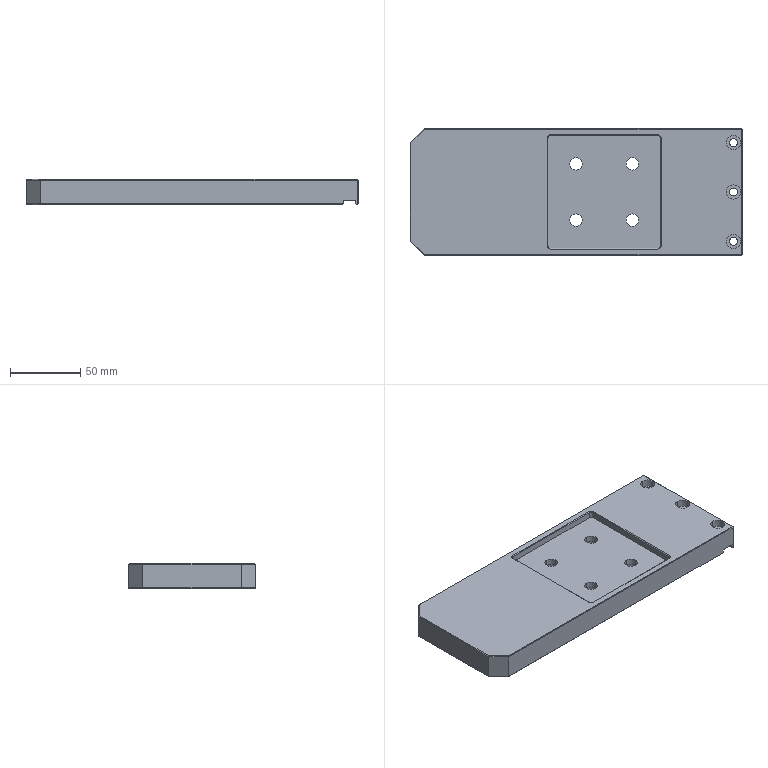NC program | NX | posted with a generic post | part box 235.5 x 90 x 18 mm
Lines 1609 to 2446 of 2446:
(ZLEVEL_PROFILE_COPY_1 , TOOL : D4)
N3186 T11 M6
N3188 G54
N3190 G17 G0 G90 X54.41 Y-37.2 S9500 M3
N3192 G43 Z30. H11
N3194 Z-0.769
N3196 G94 G1 X54.757 Y-37.8 F1000.
N3198 G3 X55.103 Y-38. R0.4
N3200 G1 X58. F2000.
N3202 Y-35.103
N3204 G3 X57.8 Y-34.757 R0.4
N3206 G1 X57.2 Y-34.41
N3208 G0 X54.41 Y-37.2 Z-1.154
N3210 G1 X54.757 Y-37.8 F1000.
N3212 G3 X55.103 Y-38. R0.4
N3214 G1 X58. F2000.
N3216 Y-35.103
N3218 G3 X57.8 Y-34.757 R0.4
N3220 G1 X57.2 Y-34.41
N3222 G0 X54.41 Y-37.2 Z-1.538
N3224 G1 X54.757 Y-37.8 F1000.
N3226 G3 X55.103 Y-38. R0.4
N3228 G1 X58. F2000.
N3230 Y-35.103
N3232 G3 X57.8 Y-34.757 R0.4
N3234 G1 X57.2 Y-34.41
N3236 G0 X54.41 Y-37.2 Z-1.923
N3238 G1 X54.757 Y-37.8 F1000.
N3240 G3 X55.103 Y-38. R0.4
N3242 G1 X58. F2000.
N3244 Y-35.103
N3246 G3 X57.8 Y-34.757 R0.4
N3248 G1 X57.2 Y-34.41
N3250 G0 X54.41 Y-37.2 Z-2.308
N3252 G1 X54.757 Y-37.8 F1000.
N3254 G3 X55.103 Y-38. R0.4
N3256 G1 X58. F2000.
N3258 Y-35.103
N3260 G3 X57.8 Y-34.757 R0.4
N3262 G1 X57.2 Y-34.41
N3264 G0 X54.41 Y-37.2 Z-2.692
N3266 G1 X54.757 Y-37.8 F1000.
N3268 G3 X55.103 Y-38. R0.4
N3270 G1 X58. F2000.
N3272 Y-35.103
N3274 G3 X57.8 Y-34.757 R0.4
N3276 G1 X57.2 Y-34.41
N3278 G0 X54.41 Y-37.2 Z-3.077
N3280 G1 X54.757 Y-37.8 F1000.
N3282 G3 X55.103 Y-38. R0.4
N3284 G1 X58. F2000.
N3286 Y-35.103
N3288 G3 X57.8 Y-34.757 R0.4
N3290 G1 X57.2 Y-34.41
N3292 G0 X54.41 Y-37.2 Z-3.462
N3294 G1 X54.757 Y-37.8 F1000.
N3296 G3 X55.103 Y-38. R0.4
N3298 G1 X58. F2000.
N3300 Y-35.103
N3302 G3 X57.8 Y-34.757 R0.4
N3304 G1 X57.2 Y-34.41
N3306 G0 X54.41 Y-37.2 Z-3.846
N3308 G1 X54.757 Y-37.8 F1000.
N3310 G3 X55.103 Y-38. R0.4
N3312 G1 X58. F2000.
N3314 Y-35.103
N3316 G3 X57.8 Y-34.757 R0.4
N3318 G1 X57.2 Y-34.41
N3320 G0 X54.41 Y-37.2 Z-4.231
N3322 G1 X54.757 Y-37.8 F1000.
N3324 G3 X55.103 Y-38. R0.4
N3326 G1 X58. F2000.
N3328 Y-35.103
N3330 G3 X57.8 Y-34.757 R0.4
N3332 G1 X57.2 Y-34.41
N3334 G0 X54.41 Y-37.2 Z-4.615
N3336 G1 X54.757 Y-37.8 F1000.
N3338 G3 X55.103 Y-38. R0.4
N3340 G1 X58. F2000.
N3342 Y-35.103
N3344 G3 X57.8 Y-34.757 R0.4
N3346 G1 X57.2 Y-34.41
N3348 G0 X54.41 Y-37.2 Z-5.
N3350 G1 X54.757 Y-37.8 F1000.
N3352 G3 X55.103 Y-38. R0.4
N3354 G1 X58. F2000.
N3356 Y-35.103
N3358 G3 X57.8 Y-34.757 R0.4
N3360 G1 X57.2 Y-34.41
N3362 G0 Z30.
N3364 Y34.41
N3366 Z-0.769
N3368 G1 X57.8 Y34.757 F1000.
N3370 G3 X58. Y35.103 R0.4
N3372 G1 Y38. F2000.
N3374 X55.103
N3376 G3 X54.757 Y37.8 R0.4
N3378 G1 X54.41 Y37.2
N3380 G0 X57.2 Y34.41 Z-1.154
N3382 G1 X57.8 Y34.757 F1000.
N3384 G3 X58. Y35.103 R0.4
N3386 G1 Y38. F2000.
N3388 X55.103
N3390 G3 X54.757 Y37.8 R0.4
N3392 G1 X54.41 Y37.2
N3394 G0 X57.2 Y34.41 Z-1.538
N3396 G1 X57.8 Y34.757 F1000.
N3398 G3 X58. Y35.103 R0.4
N3400 G1 Y38. F2000.
N3402 X55.103
N3404 G3 X54.757 Y37.8 R0.4
N3406 G1 X54.41 Y37.2
N3408 G0 X57.2 Y34.41 Z-1.923
N3410 G1 X57.8 Y34.757 F1000.
N3412 G3 X58. Y35.103 R0.4
N3414 G1 Y38. F2000.
N3416 X55.103
N3418 G3 X54.757 Y37.8 R0.4
N3420 G1 X54.41 Y37.2
N3422 G0 X57.2 Y34.41 Z-2.308
N3424 G1 X57.8 Y34.757 F1000.
N3426 G3 X58. Y35.103 R0.4
N3428 G1 Y38. F2000.
N3430 X55.103
N3432 G3 X54.757 Y37.8 R0.4
N3434 G1 X54.41 Y37.2
N3436 G0 X57.2 Y34.41 Z-2.692
N3438 G1 X57.8 Y34.757 F1000.
N3440 G3 X58. Y35.103 R0.4
N3442 G1 Y38. F2000.
N3444 X55.103
N3446 G3 X54.757 Y37.8 R0.4
N3448 G1 X54.41 Y37.2
N3450 G0 X57.2 Y34.41 Z-3.077
N3452 G1 X57.8 Y34.757 F1000.
N3454 G3 X58. Y35.103 R0.4
N3456 G1 Y38. F2000.
N3458 X55.103
N3460 G3 X54.757 Y37.8 R0.4
N3462 G1 X54.41 Y37.2
N3464 G0 X57.2 Y34.41 Z-3.462
N3466 G1 X57.8 Y34.757 F1000.
N3468 G3 X58. Y35.103 R0.4
N3470 G1 Y38. F2000.
N3472 X55.103
N3474 G3 X54.757 Y37.8 R0.4
N3476 G1 X54.41 Y37.2
N3478 G0 X57.2 Y34.41 Z-3.846
N3480 G1 X57.8 Y34.757 F1000.
N3482 G3 X58. Y35.103 R0.4
N3484 G1 Y38. F2000.
N3486 X55.103
N3488 G3 X54.757 Y37.8 R0.4
N3490 G1 X54.41 Y37.2
N3492 G0 X57.2 Y34.41 Z-4.231
N3494 G1 X57.8 Y34.757 F1000.
N3496 G3 X58. Y35.103 R0.4
N3498 G1 Y38. F2000.
N3500 X55.103
N3502 G3 X54.757 Y37.8 R0.4
N3504 G1 X54.41 Y37.2
N3506 G0 X57.2 Y34.41 Z-4.615
N3508 G1 X57.8 Y34.757 F1000.
N3510 G3 X58. Y35.103 R0.4
N3512 G1 Y38. F2000.
N3514 X55.103
N3516 G3 X54.757 Y37.8 R0.4
N3518 G1 X54.41 Y37.2
N3520 G0 X57.2 Y34.41 Z-5.
N3522 G1 X57.8 Y34.757 F1000.
N3524 G3 X58. Y35.103 R0.4
N3526 G1 Y38. F2000.
N3528 X55.103
N3530 G3 X54.757 Y37.8 R0.4
N3532 G1 X54.41 Y37.2
N3534 G0 Z30.
N3536 X-14.41
N3538 Z-0.769
N3540 G1 X-14.757 Y37.8 F1000.
N3542 G3 X-15.103 Y38. R0.4
N3544 G1 X-17.91 F2000.
N3546 X-18.
N3548 Y35.103
N3550 G3 X-17.8 Y34.757 R0.4
N3552 G1 X-17.2 Y34.41
N3554 G0 X-14.41 Y37.2 Z-1.154
N3556 G1 X-14.757 Y37.8 F1000.
N3558 G3 X-15.103 Y38. R0.4
N3560 G1 X-17.91 F2000.
N3562 X-18.
N3564 Y35.103
N3566 G3 X-17.8 Y34.757 R0.4
N3568 G1 X-17.2 Y34.41
N3570 G0 X-14.41 Y37.2 Z-1.538
N3572 G1 X-14.757 Y37.8 F1000.
N3574 G3 X-15.103 Y38. R0.4
N3576 G1 X-17.91 F2000.
N3578 X-18.
N3580 Y35.103
N3582 G3 X-17.8 Y34.757 R0.4
N3584 G1 X-17.2 Y34.41
N3586 G0 X-14.41 Y37.2 Z-1.923
N3588 G1 X-14.757 Y37.8 F1000.
N3590 G3 X-15.103 Y38. R0.4
N3592 G1 X-17.91 F2000.
N3594 X-18.
N3596 Y35.103
N3598 G3 X-17.8 Y34.757 R0.4
N3600 G1 X-17.2 Y34.41
N3602 G0 X-14.41 Y37.2 Z-2.308
N3604 G1 X-14.757 Y37.8 F1000.
N3606 G3 X-15.103 Y38. R0.4
N3608 G1 X-17.91 F2000.
N3610 X-18.
N3612 Y35.103
N3614 G3 X-17.8 Y34.757 R0.4
N3616 G1 X-17.2 Y34.41
N3618 G0 X-14.41 Y37.2 Z-2.692
N3620 G1 X-14.757 Y37.8 F1000.
N3622 G3 X-15.103 Y38. R0.4
N3624 G1 X-17.91 F2000.
N3626 X-18.
N3628 Y35.103
N3630 G3 X-17.8 Y34.757 R0.4
N3632 G1 X-17.2 Y34.41
N3634 G0 X-14.41 Y37.2 Z-3.077
N3636 G1 X-14.757 Y37.8 F1000.
N3638 G3 X-15.103 Y38. R0.4
N3640 G1 X-17.91 F2000.
N3642 X-18.
N3644 Y35.103
N3646 G3 X-17.8 Y34.757 R0.4
N3648 G1 X-17.2 Y34.41
N3650 G0 X-14.41 Y37.2 Z-3.462
N3652 G1 X-14.757 Y37.8 F1000.
N3654 G3 X-15.103 Y38. R0.4
N3656 G1 X-17.91 F2000.
N3658 X-18.
N3660 Y35.103
N3662 G3 X-17.8 Y34.757 R0.4
N3664 G1 X-17.2 Y34.41
N3666 G0 X-14.41 Y37.2 Z-3.846
N3668 G1 X-14.757 Y37.8 F1000.
N3670 G3 X-15.103 Y38. R0.4
N3672 G1 X-17.91 F2000.
N3674 X-18.
N3676 Y35.103
N3678 G3 X-17.8 Y34.757 R0.4
N3680 G1 X-17.2 Y34.41
N3682 G0 X-14.41 Y37.2 Z-4.231
N3684 G1 X-14.757 Y37.8 F1000.
N3686 G3 X-15.103 Y38. R0.4
N3688 G1 X-18. F2000.
N3690 Y35.103
N3692 G3 X-17.8 Y34.757 R0.4
N3694 G1 X-17.2 Y34.41
N3696 G0 X-14.41 Y37.2 Z-4.615
N3698 G1 X-14.757 Y37.8 F1000.
N3700 G3 X-15.103 Y38. R0.4
N3702 G1 X-18. F2000.
N3704 Y35.103
N3706 G3 X-17.8 Y34.757 R0.4
N3708 G1 X-17.2 Y34.41
N3710 G0 X-14.41 Y37.2 Z-5.
N3712 G1 X-14.757 Y37.8 F1000.
N3714 G3 X-15.103 Y38. R0.4
N3716 G1 X-18. F2000.
N3718 Y35.103
N3720 G3 X-17.8 Y34.757 R0.4
N3722 G1 X-17.2 Y34.41
N3724 G0 Z30.
N3726 Y-34.41
N3728 Z-0.769
N3730 G1 X-17.8 Y-34.757 F1000.
N3732 G3 X-18. Y-35.103 R0.4
N3734 G1 Y-37.91 F2000.
N3736 Y-38.
N3738 X-15.103
N3740 G3 X-14.757 Y-37.8 R0.4
N3742 G1 X-14.41 Y-37.2
N3744 G0 X-17.2 Y-34.41 Z-1.154
N3746 G1 X-17.8 Y-34.757 F1000.
N3748 G3 X-18. Y-35.103 R0.4
N3750 G1 Y-37.91 F2000.
N3752 Y-38.
N3754 X-15.103
N3756 G3 X-14.757 Y-37.8 R0.4
N3758 G1 X-14.41 Y-37.2
N3760 G0 X-17.2 Y-34.41 Z-1.538
N3762 G1 X-17.8 Y-34.757 F1000.
N3764 G3 X-18. Y-35.103 R0.4
N3766 G1 Y-37.91 F2000.
N3768 Y-38.
N3770 X-15.103
N3772 G3 X-14.757 Y-37.8 R0.4
N3774 G1 X-14.41 Y-37.2
N3776 G0 X-17.2 Y-34.41 Z-1.923
N3778 G1 X-17.8 Y-34.757 F1000.
N3780 G3 X-18. Y-35.103 R0.4
N3782 G1 Y-37.91 F2000.
N3784 Y-38.
N3786 X-15.103
N3788 G3 X-14.757 Y-37.8 R0.4
N3790 G1 X-14.41 Y-37.2
N3792 G0 X-17.2 Y-34.41 Z-2.308
N3794 G1 X-17.8 Y-34.757 F1000.
N3796 G3 X-18. Y-35.103 R0.4
N3798 G1 Y-37.91 F2000.
N3800 Y-38.
N3802 X-15.103
N3804 G3 X-14.757 Y-37.8 R0.4
N3806 G1 X-14.41 Y-37.2
N3808 G0 X-17.2 Y-34.41 Z-2.692
N3810 G1 X-17.8 Y-34.757 F1000.
N3812 G3 X-18. Y-35.103 R0.4
N3814 G1 Y-37.91 F2000.
N3816 Y-38.
N3818 X-15.103
N3820 G3 X-14.757 Y-37.8 R0.4
N3822 G1 X-14.41 Y-37.2
N3824 G0 X-17.2 Y-34.41 Z-3.077
N3826 G1 X-17.8 Y-34.757 F1000.
N3828 G3 X-18. Y-35.103 R0.4
N3830 G1 Y-37.91 F2000.
N3832 Y-38.
N3834 X-15.103
N3836 G3 X-14.757 Y-37.8 R0.4
N3838 G1 X-14.41 Y-37.2
N3840 G0 X-17.2 Y-34.41 Z-3.462
N3842 G1 X-17.8 Y-34.757 F1000.
N3844 G3 X-18. Y-35.103 R0.4
N3846 G1 Y-37.91 F2000.
N3848 Y-38.
N3850 X-15.103
N3852 G3 X-14.757 Y-37.8 R0.4
N3854 G1 X-14.41 Y-37.2
N3856 G0 X-17.2 Y-34.41 Z-3.846
N3858 G1 X-17.8 Y-34.757 F1000.
N3860 G3 X-18. Y-35.103 R0.4
N3862 G1 Y-37.91 F2000.
N3864 Y-38.
N3866 X-15.103
N3868 G3 X-14.757 Y-37.8 R0.4
N3870 G1 X-14.41 Y-37.2
N3872 G0 X-17.2 Y-34.41 Z-4.231
N3874 G1 X-17.8 Y-34.757 F1000.
N3876 G3 X-18. Y-35.103 R0.4
N3878 G1 Y-38. F2000.
N3880 X-15.103
N3882 G3 X-14.757 Y-37.8 R0.4
N3884 G1 X-14.41 Y-37.2
N3886 G0 X-17.2 Y-34.41 Z-4.615
N3888 G1 X-17.8 Y-34.757 F1000.
N3890 G3 X-18. Y-35.103 R0.4
N3892 G1 Y-38. F2000.
N3894 X-15.103
N3896 G3 X-14.757 Y-37.8 R0.4
N3898 G1 X-14.41 Y-37.2
N3900 G0 X-17.2 Y-34.41 Z-5.
N3902 G1 X-17.8 Y-34.757 F1000.
N3904 G3 X-18. Y-35.103 R0.4
N3906 G1 Y-38. F2000.
N3908 X-15.103
N3910 G3 X-14.757 Y-37.8 R0.4
N3912 G1 X-14.41 Y-37.2
N3914 G0 Z30.
N3916 M5
(PLANAR_MILL , TOOL : D6A45)
N3918 T01 M6
N3920 G54
N3922 G17 G0 G90 X1.029 Y-17.182 S9500 M3
N3924 G43 Z30. H1
N3926 Z-5.
N3928 G94 G1 Z-6. F1500.
N3930 X0.866 Y-16.9
N3932 G3 X0. Y-16.4 R1.
N3934 X-3.6 Y-20. R3.6
N3936 X0. Y-16.4 R-3.6
N3938 X-0.866 Y-16.9 R1.
N3940 G1 X-1.029 Y-17.182
N3942 Z-5.
N3944 G0 Z30.
N3946 X38.971 Y-22.818
N3948 Z-5.
N3950 G1 Z-6.
N3952 X39.134 Y-23.1
N3954 G3 X40. Y-23.6 R1.
N3956 X43.6 Y-20. R3.6
N3958 X40. Y-23.6 R-3.6
N3960 X40.866 Y-23.1 R1.
N3962 G1 X41.029 Y-22.818
N3964 Z-5.
N3966 G0 Z30.
N3968 X38.971 Y17.182
N3970 Z-5.
N3972 G1 Z-6.
N3974 X39.134 Y16.9
N3976 G3 X40. Y16.4 R1.
N3978 X43.6 Y20. R3.6
N3980 X40. Y16.4 R-3.6
N3982 X40.866 Y16.9 R1.
N3984 G1 X41.029 Y17.182
N3986 Z-5.
N3988 G0 Z30.
N3990 X-1.029
N3992 Z-5.
N3994 G1 Z-6.
N3996 X-0.866 Y16.9
N3998 G3 X0. Y16.4 R1.
N4000 X3.6 Y20. R3.6
N4002 X0. Y16.4 R-3.6
N4004 X0.866 Y16.9 R1.
N4006 G1 X1.029 Y17.182
N4008 Z-5.
N4010 G0 Z30.
(PLANAR_MILL_COPY , TOOL : D6A45)
N4012 X112.76 Y38.351
N4014 Z0.
N4016 G1 Z-1.
N4018 X112.616 Y38.6
N4020 G3 X111.75 Y39.1 R1.
N4022 X107.65 Y35. R4.1
N4024 X111.75 Y39.1 R-4.1
N4026 X110.884 Y38.6 R1.
N4028 G1 X110.74 Y38.351
N4030 Z0.
N4032 G0 Z30.
N4034 Y-3.351
N4036 Z0.
N4038 G1 Z-1.
N4040 X110.884 Y-3.6
N4042 G3 X111.75 Y-4.1 R1.
N4044 X115.85 Y0. R4.1
N4046 X111.75 Y-4.1 R-4.1
N4048 X112.616 Y-3.6 R1.
N4050 G1 X112.76 Y-3.351
N4052 Z0.
N4054 G0 Z30.
N4056 X110.74 Y-38.351
N4058 Z0.
N4060 G1 Z-1.
N4062 X110.884 Y-38.6
N4064 G3 X111.75 Y-39.1 R1.
N4066 X115.85 Y-35. R4.1
N4068 X111.75 Y-39.1 R-4.1
N4070 X112.616 Y-38.6 R1.
N4072 G1 X112.76 Y-38.351
N4074 Z0.
N4076 G0 Z30.
(PLANAR_MILL_COPY_COPY , TOOL : D6A45)
N4078 X3.988 Y46.
N4080 Z0.
N4082 G1 Z-1.
N4084 G3 X4.854 Y45.5 R1.
N4086 G1 X117.25
N4088 G2 X118.25 Y44.5 R1.
N4090 G1 Y-44.5
N4092 G2 X117.25 Y-45.5 R1.
N4094 G1 X-107.543
N4096 G2 X-108.25 Y-45.207 R1.
N4098 G1 X-117.957 Y-35.5
N4100 G2 X-118.25 Y-34.793 R1.
N4102 G1 Y34.793
N4104 G2 X-117.957 Y35.5 R1.
N4106 G1 X-108.25 Y45.207
N4108 G2 X-107.543 Y45.5 R1.
N4110 G1 X4.854
N4112 G3 X5.72 Y46. R1.
N4114 G1 Z0.
N4116 G0 Z30.
N4118 X20.866 Y39.
N4120 Z0.
N4122 G1 Z-1.
N4124 G3 X20. Y39.5 R1.
N4126 G1 X-18.
N4128 G3 X-19.5 Y38. R1.5
N4130 G1 Y-38.
N4132 G3 X-18. Y-39.5 R1.5
N4134 G1 X58.
N4136 G3 X59.5 Y-38. R1.5
N4138 G1 Y38.
N4140 G3 X58. Y39.5 R1.5
N4142 G1 X20.
N4144 G3 X19.134 Y39. R1.
N4146 G1 Z0.
N4148 G0 Z30.
N4150 M5
(FLOOR_WALL_COPY , TOOL : D10JING)
N4152 T14 M6
N4154 G54
N4156 G17 G0 G90 X18.378 Y-4.5 S9500 M3
N4158 G43 Z30. H14
N4160 Z-3.5
N4162 G94 G1 X24.5 Z-3.821 F1000.
N4164 Y4.5 Z-4.292
N4166 X15.5 Z-4.764
N4168 Y0. Z-5.
N4170 X20.
N4172 X15.5 F1500.
N4174 Y-4.5
N4176 X24.5
N4178 Y4.5
N4180 X15.5
N4182 Y0.
N4184 X10.5
N4186 Y-9.5
N4188 X29.5
N4190 Y9.5
N4192 X10.5
N4194 Y0.
N4196 X5.5
N4198 Y-14.5
N4200 X34.5
N4202 Y14.5
N4204 X5.5
N4206 Y0.
N4208 X0.5
N4210 Y-19.5
N4212 X39.5
N4214 Y19.5
N4216 X0.5
N4218 Y0.
N4220 X-4.5
N4222 Y-24.5
N4224 X44.5
N4226 Y24.5
N4228 X-4.5
N4230 Y0.
N4232 X-9.5
N4234 Y-29.5
N4236 X49.5
N4238 Y29.5
N4240 X-9.5
N4242 Y0.
N4244 X-14.5
N4246 Y-34.5
N4248 X54.5
N4250 Y34.5
N4252 X-14.5
N4254 Y0.
N4256 Z-3.5
N4258 G0 Z-1.9
N4260 X-15. Y28.622
N4262 Z-3.5
N4264 G1 Y0. Z-5. F1000.
N4266 Y-35. F1500.
N4268 X55.
N4270 Y35.
N4272 X-15.
N4274 Y0.
N4276 Z-3.5
N4278 G0 Z30.
(ZLEVEL_PROFILE_COPY , TOOL : D10JING)
N4280 X122.75 Y-36.738
N4282 Z1.1
N4284 G1 Y-45.049 Z0.664 F1000.
N4286 X122.397 Y-46.425 Z0.59
N4288 X121.673 Y-47.648 Z0.516
N4290 X120.398 Y-48.923 Z0.421
N4292 X119.175 Y-49.647 Z0.347
N4294 X117.799 Y-50. Z0.272
N4296 X-108.299 Z-11.577
N4298 X-109.675 Y-49.647 Z-11.652
N4300 X-110.898 Y-48.923 Z-11.726
N4302 X-121.673 Y-38.148 Z-12.525
N4304 X-122.397 Y-36.925 Z-12.599
N4306 X-122.75 Y-35.549 Z-12.674
N4308 Y35.549 Z-16.4
N4310 X-122.397 Y36.925 Z-16.474
N4312 X-121.673 Y38.148 Z-16.549
N4314 X-110.898 Y48.923 Z-17.347
N4316 X-109.675 Y49.647 Z-17.422
N4318 X-108.299 Y50. Z-17.496
N4320 X-107.75 Z-17.525
N4322 X117.25 F1500.
N4324 G2 X120.786 Y48.536 R5.
N4326 G1 X121.286 Y48.036
N4328 G2 X122.75 Y44.5 R5.
N4330 G1 Y-44.5
N4332 G2 X121.286 Y-48.036 R5.
N4334 G1 X120.786 Y-48.536
N4336 G2 X117.25 Y-50. R5.
N4338 G1 X-107.75
N4340 G2 X-111.286 Y-48.536 R5.
N4342 G1 X-121.286 Y-38.536
N4344 G2 X-122.75 Y-35. R5.
N4346 G1 Y35.
N4348 G2 X-121.286 Y38.536 R5.
N4350 G1 X-111.286 Y48.536
N4352 G2 X-107.75 Y50. R5.
N4354 G1 X117.25 Z-17.567
N4356 X117.74 Y49.976
N4358 X118.225 Y49.904
N4360 X118.701 Y49.785
N4362 X119.163 Y49.619
N4364 X119.607 Y49.41
N4366 X120.028 Y49.157 Z-17.568
N4368 X120.422 Y48.865
N4370 X120.786 Y48.536
N4372 X121.286 Y48.036
N4374 X121.615 Y47.672
N4376 X121.907 Y47.278
N4378 X122.16 Y46.857
N4380 X122.369 Y46.413
N4382 X122.535 Y45.951
N4384 X122.654 Y45.475
N4386 X122.726 Y44.99
N4388 X122.75 Y44.5 Z-17.569
N4390 Y-44.5 Z-17.585
N4392 X122.726 Y-44.99
N4394 X122.654 Y-45.475
N4396 X122.535 Y-45.951
N4398 X122.369 Y-46.413 Z-17.586
N4400 X122.16 Y-46.857
N4402 X121.907 Y-47.278
N4404 X121.615 Y-47.672
N4406 X121.286 Y-48.036
N4408 X120.786 Y-48.536
N4410 X120.422 Y-48.865
N4412 X120.028 Y-49.157
N4414 X119.607 Y-49.41
N4416 X119.163 Y-49.619
N4418 X118.701 Y-49.785
N4420 X118.225 Y-49.904 Z-17.587
N4422 X117.74 Y-49.976
N4424 X117.25 Y-50.
N4426 X-107.75 Z-17.629
N4428 X-108.24 Y-49.976
N4430 X-108.725 Y-49.904
N4432 X-109.201 Y-49.785
N4434 X-109.663 Y-49.619
N4436 X-110.107 Y-49.41
N4438 X-110.528 Y-49.157
N4440 X-110.922 Y-48.865
N4442 X-111.286 Y-48.536
N4444 X-121.286 Y-38.536 Z-17.632
N4446 X-121.615 Y-38.172
N4448 X-121.907 Y-37.778
N4450 X-122.16 Y-37.357
N4452 X-122.369 Y-36.913
N4454 X-122.535 Y-36.451 Z-17.633
N4456 X-122.654 Y-35.975
N4458 X-122.726 Y-35.49
N4460 X-122.75 Y-35.
N4462 Y35. Z-17.646
N4464 X-122.726 Y35.49
N4466 X-122.654 Y35.975
N4468 X-122.535 Y36.451
N4470 X-122.369 Y36.913
N4472 X-122.16 Y37.357
N4474 X-121.907 Y37.778
N4476 X-121.615 Y38.172 Z-17.647
N4478 X-121.286 Y38.536
N4480 X-111.286 Y48.536 Z-17.649
N4482 X-110.922 Y48.865
N4484 X-110.528 Y49.157
N4486 X-110.107 Y49.41 Z-17.65
N4488 X-109.663 Y49.619
N4490 X-109.201 Y49.785
N4492 X-108.725 Y49.904
N4494 X-108.24 Y49.976
N4496 X-107.75 Y50.
N4498 X117.25 Z-17.692
N4500 X117.74 Y49.976
N4502 X118.225 Y49.904
N4504 X118.701 Y49.785
N4506 X119.163 Y49.619
N4508 X119.607 Y49.41
N4510 X120.028 Y49.157 Z-17.693
N4512 X120.422 Y48.865
N4514 X120.786 Y48.536
N4516 X121.286 Y48.036
N4518 X121.615 Y47.672
N4520 X121.907 Y47.278
N4522 X122.16 Y46.857
N4524 X122.369 Y46.413
N4526 X122.535 Y45.951
N4528 X122.654 Y45.475
N4530 X122.726 Y44.99
N4532 X122.75 Y44.5 Z-17.694
N4534 Y-44.5 Z-17.71
N4536 X122.726 Y-44.99
N4538 X122.654 Y-45.475
N4540 X122.535 Y-45.951
N4542 X122.369 Y-46.413 Z-17.711
N4544 X122.16 Y-46.857
N4546 X121.907 Y-47.278
N4548 X121.615 Y-47.672
N4550 X121.286 Y-48.036
N4552 X120.786 Y-48.536
N4554 X120.422 Y-48.865
N4556 X120.028 Y-49.157
N4558 X119.607 Y-49.41
N4560 X119.163 Y-49.619
N4562 X118.701 Y-49.785
N4564 X118.225 Y-49.904 Z-17.712
N4566 X117.74 Y-49.976
N4568 X117.25 Y-50.
N4570 X-107.75 Z-17.754
N4572 X-108.24 Y-49.976
N4574 X-108.725 Y-49.904
N4576 X-109.201 Y-49.785
N4578 X-109.663 Y-49.619
N4580 X-110.107 Y-49.41
N4582 X-110.528 Y-49.157
N4584 X-110.922 Y-48.865
N4586 X-111.286 Y-48.536
N4588 X-121.286 Y-38.536 Z-17.757
N4590 X-121.615 Y-38.172
N4592 X-121.907 Y-37.778
N4594 X-122.16 Y-37.357
N4596 X-122.369 Y-36.913
N4598 X-122.535 Y-36.451 Z-17.758
N4600 X-122.654 Y-35.975
N4602 X-122.726 Y-35.49
N4604 X-122.75 Y-35.
N4606 Y35. Z-17.771
N4608 X-122.726 Y35.49
N4610 X-122.654 Y35.975
N4612 X-122.535 Y36.451
N4614 X-122.369 Y36.913
N4616 X-122.16 Y37.357
N4618 X-121.907 Y37.778
N4620 X-121.615 Y38.172 Z-17.772
N4622 X-121.286 Y38.536
N4624 X-111.286 Y48.536 Z-17.774
N4626 X-110.922 Y48.865
N4628 X-110.528 Y49.157
N4630 X-110.107 Y49.41 Z-17.775
N4632 X-109.663 Y49.619
N4634 X-109.201 Y49.785
N4636 X-108.725 Y49.904
N4638 X-108.24 Y49.976
N4640 X-107.75 Y50.
N4642 X117.25 Z-17.817
N4644 X117.74 Y49.976
N4646 X118.225 Y49.904
N4648 X118.701 Y49.785
N4650 X119.163 Y49.619
N4652 X119.607 Y49.41
N4654 X120.028 Y49.157 Z-17.818
N4656 X120.422 Y48.865
N4658 X120.786 Y48.536
N4660 X121.286 Y48.036
N4662 X121.615 Y47.672
N4664 X121.907 Y47.278
N4666 X122.16 Y46.857
N4668 X122.369 Y46.413
N4670 X122.535 Y45.951
N4672 X122.654 Y45.475
N4674 X122.726 Y44.99
N4676 X122.75 Y44.5 Z-17.819
N4678 Y-44.5 Z-17.835
N4680 X122.726 Y-44.99
N4682 X122.654 Y-45.475
N4684 X122.535 Y-45.951
N4686 X122.369 Y-46.413 Z-17.836
N4688 X122.16 Y-46.857
N4690 X121.907 Y-47.278
N4692 X121.615 Y-47.672
N4694 X121.286 Y-48.036
N4696 X120.786 Y-48.536
N4698 X120.422 Y-48.865
N4700 X120.028 Y-49.157
N4702 X119.607 Y-49.41
N4704 X119.163 Y-49.619
N4706 X118.701 Y-49.785
N4708 X118.225 Y-49.904 Z-17.837
N4710 X117.74 Y-49.976
N4712 X117.25 Y-50.
N4714 X-107.75 Z-17.879
N4716 X-108.24 Y-49.976
N4718 X-108.725 Y-49.904
N4720 X-109.201 Y-49.785
N4722 X-109.663 Y-49.619
N4724 X-110.107 Y-49.41
N4726 X-110.528 Y-49.157
N4728 X-110.922 Y-48.865
N4730 X-111.286 Y-48.536
N4732 X-121.286 Y-38.536 Z-17.882
N4734 X-121.615 Y-38.172
N4736 X-121.907 Y-37.778
N4738 X-122.16 Y-37.357
N4740 X-122.369 Y-36.913
N4742 X-122.535 Y-36.451 Z-17.883
N4744 X-122.654 Y-35.975
N4746 X-122.726 Y-35.49
N4748 X-122.75 Y-35.
N4750 Y35. Z-17.896
N4752 X-122.726 Y35.49
N4754 X-122.654 Y35.975
N4756 X-122.535 Y36.451
N4758 X-122.369 Y36.913
N4760 X-122.16 Y37.357
N4762 X-121.907 Y37.778
N4764 X-121.615 Y38.172 Z-17.897
N4766 X-121.286 Y38.536
N4768 X-111.286 Y48.536 Z-17.899
N4770 X-110.922 Y48.865
N4772 X-110.528 Y49.157
N4774 X-110.107 Y49.41 Z-17.9
N4776 X-109.663 Y49.619
N4778 X-109.201 Y49.785
N4780 X-108.725 Y49.904
N4782 X-108.24 Y49.976
N4784 X-107.75 Y50.
N4786 X117.25
N4788 G2 X120.786 Y48.536 R5.
N4790 G1 X121.286 Y48.036
N4792 G2 X122.75 Y44.5 R5.
N4794 G1 Y-44.5
N4796 G2 X121.286 Y-48.036 R5.
N4798 G1 X120.786 Y-48.536
N4800 G2 X117.25 Y-50. R5.
N4802 G1 X-107.75
N4804 G2 X-111.286 Y-48.536 R5.
N4806 G1 X-121.286 Y-38.536
N4808 G2 X-122.75 Y-35. R5.
N4810 G1 Y35.
N4812 G2 X-121.286 Y38.536 R5.
N4814 G1 X-111.286 Y48.536
N4816 G2 X-107.75 Y50. R5.
N4818 G1 Z0.6
N4820 G0 Z30.
N4822 M5
N4824 M2